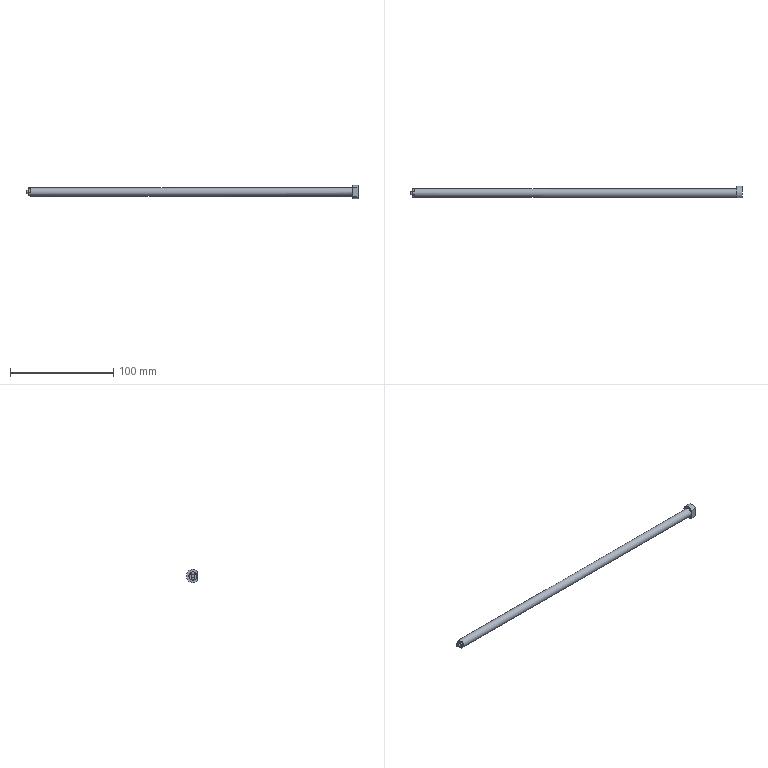Part | STEP file | solid 255 | 1 solid | 23 faces | box 322.109 x 11 x 13 mm | volume 16427 mm3 | spline 12 | plane 9 | cylinder 2 | commonest cylinder face diameters 8 x1 13 x1